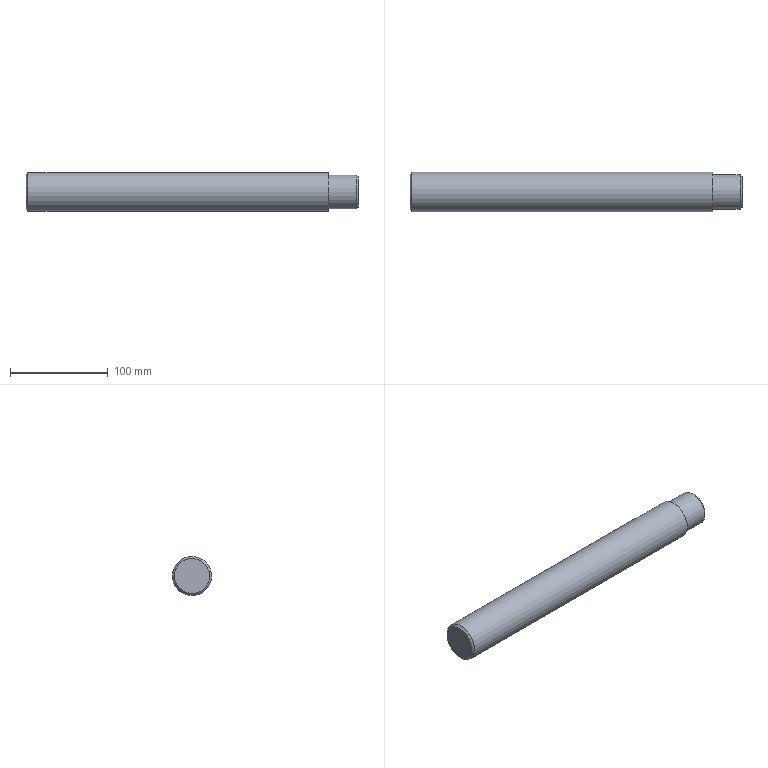Part | NX | features 00 2 | 1 solid | 7 faces | box 340 x 40 x 40 mm | volume 417966 mm3 | plane 3 | cone 2 | cylinder 2 | commonest cylinder face diameters 35 x1 40 x1
STEP:
#1=CARTESIAN_POINT('',(131.7,-103.501,-820.317));
#2=VERTEX_POINT('',#1);
#3=CARTESIAN_POINT('',(131.7,-119.,-820.129));
#4=DIRECTION('',(1.,0.,0.));
#5=DIRECTION('',(0.,0.9999,-0.01213));
#6=AXIS2_PLACEMENT_3D('',#3,#4,#5);
#7=CIRCLE('',#6,15.5);
#8=EDGE_CURVE('',#2,#2,#7,.T.);
#9=ORIENTED_EDGE('',*,*,#8,.T.);
#10=EDGE_LOOP('',(#9));
#11=FACE_BOUND('',#10,.T.);
#12=CARTESIAN_POINT('',(131.7,-118.788,-802.631));
#13=DIRECTION('',(-1.,0.,0.));
#14=DIRECTION('',(0.,-0.9999,0.01213));
#15=AXIS2_PLACEMENT_3D('',#12,#13,#14);
#16=PLANE('',#15);
#17=ADVANCED_FACE('',(#11),#16,.F.);
#18=ORIENTED_EDGE('',*,*,#8,.F.);
#19=EDGE_LOOP('',(#18));
#20=FACE_BOUND('',#19,.T.);
#21=CARTESIAN_POINT('',(129.7,-101.501,-820.342));
#22=VERTEX_POINT('',#21);
#23=CARTESIAN_POINT('',(129.7,-119.,-820.129));
#24=DIRECTION('',(1.,0.,0.));
#25=DIRECTION('',(0.,0.9999,-0.01213));
#26=AXIS2_PLACEMENT_3D('',#23,#24,#25);
#27=CIRCLE('',#26,17.5);
#28=EDGE_CURVE('',#22,#22,#27,.T.);
#29=ORIENTED_EDGE('',*,*,#28,.T.);
#30=EDGE_LOOP('',(#29));
#31=FACE_BOUND('',#30,.T.);
#32=CARTESIAN_POINT('',(131.992,-119.,-820.129));
#33=DIRECTION('',(-1.,0.,0.));
#34=DIRECTION('',(0.,-0.9999,0.01213));
#35=AXIS2_PLACEMENT_3D('',#32,#33,#34);
#36=CONICAL_SURFACE('',#35,15.208,0.7854);
#37=ADVANCED_FACE('',(#20,#31),#36,.T.);
#38=CARTESIAN_POINT('',(101.7,-136.499,-819.917));
#39=VERTEX_POINT('',#38);
#40=CARTESIAN_POINT('',(101.7,-119.,-820.129));
#41=DIRECTION('',(-1.,0.,0.));
#42=DIRECTION('',(0.,-0.9999,0.01213));
#43=AXIS2_PLACEMENT_3D('',#40,#41,#42);
#44=CIRCLE('',#43,17.5);
#45=EDGE_CURVE('',#39,#39,#44,.T.);
#46=ORIENTED_EDGE('',*,*,#45,.F.);
#47=EDGE_LOOP('',(#46));
#48=FACE_BOUND('',#47,.T.);
#49=ORIENTED_EDGE('',*,*,#28,.F.);
#50=EDGE_LOOP('',(#49));
#51=FACE_BOUND('',#50,.T.);
#52=CARTESIAN_POINT('',(-208.3,-119.,-820.129));
#53=DIRECTION('',(-1.,0.,0.));
#54=DIRECTION('',(0.,-0.9999,0.01213));
#55=AXIS2_PLACEMENT_3D('',#52,#53,#54);
#56=CYLINDRICAL_SURFACE('',#55,17.5);
#57=ADVANCED_FACE('',(#48,#51),#56,.T.);
#58=ORIENTED_EDGE('',*,*,#45,.T.);
#59=EDGE_LOOP('',(#58));
#60=FACE_BOUND('',#59,.T.);
#61=CARTESIAN_POINT('',(101.7,-99.001,-820.372));
#62=VERTEX_POINT('',#61);
#63=CARTESIAN_POINT('',(101.7,-119.,-820.129));
#64=DIRECTION('',(1.,0.,0.));
#65=DIRECTION('',(0.,0.9999,-0.01213));
#66=AXIS2_PLACEMENT_3D('',#63,#64,#65);
#67=CIRCLE('',#66,20.);
#68=EDGE_CURVE('',#62,#62,#67,.T.);
#69=ORIENTED_EDGE('',*,*,#68,.T.);
#70=EDGE_LOOP('',(#69));
#71=FACE_BOUND('',#70,.T.);
#72=CARTESIAN_POINT('',(101.7,-118.757,-800.131));
#73=DIRECTION('',(-1.,0.,0.));
#74=DIRECTION('',(0.,-0.9999,0.01213));
#75=AXIS2_PLACEMENT_3D('',#72,#73,#74);
#76=PLANE('',#75);
#77=ADVANCED_FACE('',(#60,#71),#76,.F.);
#78=CARTESIAN_POINT('',(-206.3,-99.001,-820.372));
#79=VERTEX_POINT('',#78);
#80=CARTESIAN_POINT('',(-206.3,-119.,-820.129));
#81=DIRECTION('',(-1.,0.,0.));
#82=DIRECTION('',(0.,0.9999,-0.01213));
#83=AXIS2_PLACEMENT_3D('',#80,#81,#82);
#84=CIRCLE('',#83,20.);
#85=EDGE_CURVE('',#79,#79,#84,.T.);
#86=ORIENTED_EDGE('',*,*,#85,.F.);
#87=EDGE_LOOP('',(#86));
#88=FACE_BOUND('',#87,.T.);
#89=ORIENTED_EDGE('',*,*,#68,.F.);
#90=EDGE_LOOP('',(#89));
#91=FACE_BOUND('',#90,.T.);
#92=CARTESIAN_POINT('',(-208.3,-119.,-820.129));
#93=DIRECTION('',(-1.,0.,0.));
#94=DIRECTION('',(0.,-0.9999,0.01213));
#95=AXIS2_PLACEMENT_3D('',#92,#93,#94);
#96=CYLINDRICAL_SURFACE('',#95,20.);
#97=ADVANCED_FACE('',(#88,#91),#96,.T.);
#98=CARTESIAN_POINT('',(-208.3,-101.001,-820.348));
#99=VERTEX_POINT('',#98);
#100=CARTESIAN_POINT('',(-208.3,-119.,-820.129));
#101=DIRECTION('',(-1.,0.,0.));
#102=DIRECTION('',(0.,0.9999,-0.01213));
#103=AXIS2_PLACEMENT_3D('',#100,#101,#102);
#104=CIRCLE('',#103,18.);
#105=EDGE_CURVE('',#99,#99,#104,.T.);
#106=ORIENTED_EDGE('',*,*,#105,.T.);
#107=EDGE_LOOP('',(#106));
#108=FACE_BOUND('',#107,.T.);
#109=CARTESIAN_POINT('',(-208.3,-119.,-820.129));
#110=DIRECTION('',(1.,0.,0.));
#111=DIRECTION('',(0.,0.9999,-0.01213));
#112=AXIS2_PLACEMENT_3D('',#109,#110,#111);
#113=PLANE('',#112);
#114=ADVANCED_FACE('',(#108),#113,.F.);
#115=ORIENTED_EDGE('',*,*,#105,.F.);
#116=EDGE_LOOP('',(#115));
#117=FACE_BOUND('',#116,.T.);
#118=ORIENTED_EDGE('',*,*,#85,.T.);
#119=EDGE_LOOP('',(#118));
#120=FACE_BOUND('',#119,.T.);
#121=CARTESIAN_POINT('',(-208.592,-119.,-820.129));
#122=DIRECTION('',(1.,0.,0.));
#123=DIRECTION('',(0.,0.9999,-0.01213));
#124=AXIS2_PLACEMENT_3D('',#121,#122,#123);
#125=CONICAL_SURFACE('',#124,17.708,0.7854);
#126=ADVANCED_FACE('',(#117,#120),#125,.T.);
#127=CLOSED_SHELL('',(#17,#37,#57,#77,#97,#114,#126));
#128=MANIFOLD_SOLID_BREP('',#127);
#129=(LENGTH_UNIT()NAMED_UNIT(*)SI_UNIT(.MILLI.,.METRE.));
#130=UNCERTAINTY_MEASURE_WITH_UNIT(LENGTH_MEASURE(0.00001),#129,'','');
#131=(NAMED_UNIT(*)PLANE_ANGLE_UNIT()SI_UNIT($,.RADIAN.));
#132=(NAMED_UNIT(*)SI_UNIT($,.STERADIAN.)SOLID_ANGLE_UNIT());
#133=(GEOMETRIC_REPRESENTATION_CONTEXT(3)GLOBAL_UNCERTAINTY_ASSIGNED_CONTEXT((#130))GLOBAL_UNIT_ASSIGNED_CONTEXT((#129,#131,#132))REPRESENTATION_CONTEXT('',''));
#134=ADVANCED_BREP_SHAPE_REPRESENTATION('',(#128),#133);